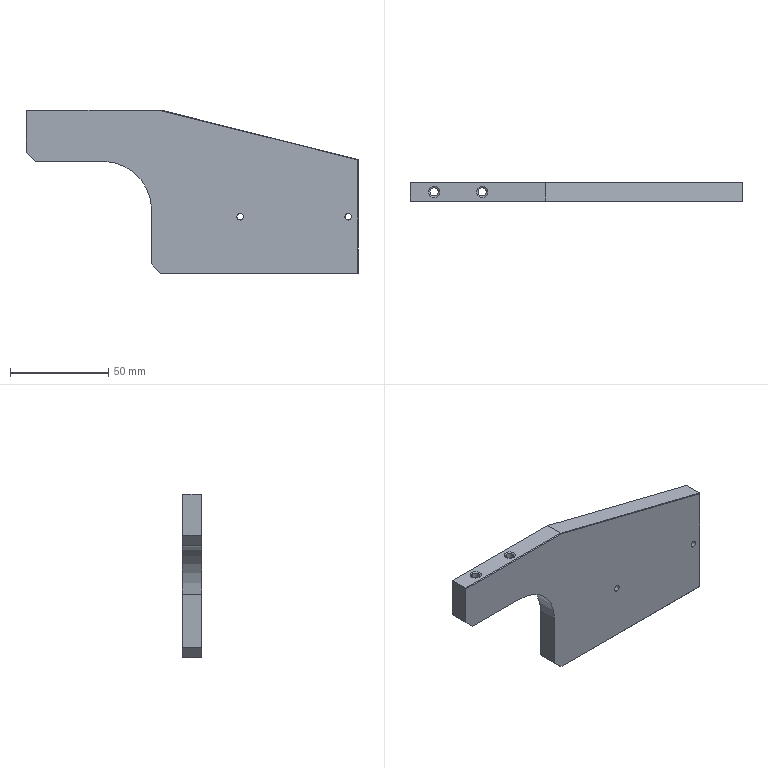Part | NX | 1 solid | 56 faces | box 169 x 10 x 83.25 mm | volume 91620 mm3 | plane 23 | cylinder 17 | cone 16 | commonest cylinder face diameters 2.5 x8 3.3 x4 4.2 x4 50 x1